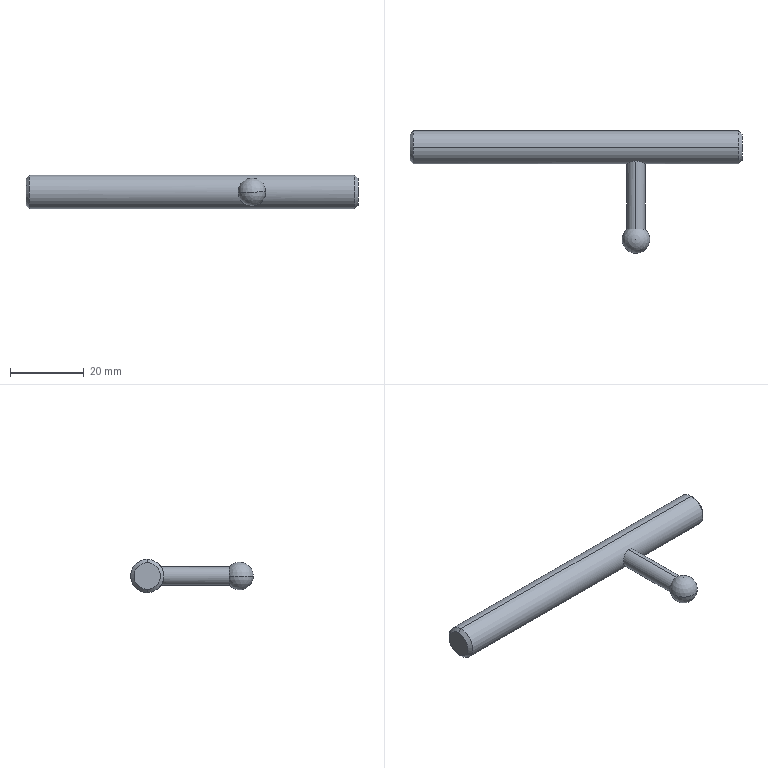Part | SolidWorks | features BaseBody 1 | 1 solid | 12 faces | box 90 x 33.25 x 9 mm | volume 6266 mm3 | cylinder 4 | cone 4 | sphere 2 | plane 2 | commonest cylinder face diameters 5 x2 9 x2
STEP:
#1=CARTESIAN_POINT('',(37.5,-25.,5.7));
#2=VERTEX_POINT('',#1);
#3=CARTESIAN_POINT('',(45.,-25.,5.7));
#4=VERTEX_POINT('',#3);
#5=CARTESIAN_POINT('',(41.25,-25.,5.7));
#6=DIRECTION('',(0.,0.,1.));
#7=DIRECTION('',(1.,0.,0.));
#8=AXIS2_PLACEMENT_3D('',#5,#6,#7);
#9=CIRCLE('',#8,3.75);
#10=EDGE_CURVE('',#2,#4,#9,.T.);
#11=ORIENTED_EDGE('',*,*,#10,.F.);
#12=CARTESIAN_POINT('',(38.75,-22.205,5.7));
#13=VERTEX_POINT('',#12);
#14=CARTESIAN_POINT('',(41.25,-25.,5.7));
#15=DIRECTION('',(0.,0.,-1.));
#16=DIRECTION('',(-1.,0.,0.));
#17=AXIS2_PLACEMENT_3D('',#14,#15,#16);
#18=CIRCLE('',#17,3.75);
#19=EDGE_CURVE('',#2,#13,#18,.T.);
#20=ORIENTED_EDGE('',*,*,#19,.T.);
#21=CARTESIAN_POINT('',(41.25,-22.205,3.2));
#22=VERTEX_POINT('',#21);
#23=CARTESIAN_POINT('',(41.25,-22.205,5.7));
#24=DIRECTION('',(0.,1.,0.));
#25=DIRECTION('',(0.,0.,-1.));
#26=AXIS2_PLACEMENT_3D('',#23,#24,#25);
#27=CIRCLE('',#26,2.5);
#28=EDGE_CURVE('',#22,#13,#27,.T.);
#29=ORIENTED_EDGE('',*,*,#28,.F.);
#30=CARTESIAN_POINT('',(43.75,-22.205,5.7));
#31=VERTEX_POINT('',#30);
#32=CARTESIAN_POINT('',(41.25,-22.205,5.7));
#33=DIRECTION('',(0.,1.,0.));
#34=DIRECTION('',(0.,0.,-1.));
#35=AXIS2_PLACEMENT_3D('',#32,#33,#34);
#36=CIRCLE('',#35,2.5);
#37=EDGE_CURVE('',#31,#22,#36,.T.);
#38=ORIENTED_EDGE('',*,*,#37,.F.);
#39=CARTESIAN_POINT('',(41.25,-25.,5.7));
#40=DIRECTION('',(0.,0.,-1.));
#41=DIRECTION('',(-1.,0.,0.));
#42=AXIS2_PLACEMENT_3D('',#39,#40,#41);
#43=CIRCLE('',#42,3.75);
#44=EDGE_CURVE('',#31,#4,#43,.T.);
#45=ORIENTED_EDGE('',*,*,#44,.T.);
#46=EDGE_LOOP('',(#11,#20,#29,#38,#45));
#47=FACE_OUTER_BOUND('',#46,.T.);
#48=CARTESIAN_POINT('',(41.25,-25.,5.7));
#49=DIRECTION('',(0.,0.,-1.));
#50=DIRECTION('',(0.,-1.,0.));
#51=AXIS2_PLACEMENT_3D('',#48,#49,#50);
#52=SPHERICAL_SURFACE('',#51,3.75);
#53=ADVANCED_FACE('',(#47),#52,.T.);
#54=CARTESIAN_POINT('',(-19.1,0.,1.2));
#55=VERTEX_POINT('',#54);
#56=CARTESIAN_POINT('',(-19.1,0.,10.2));
#57=VERTEX_POINT('',#56);
#58=CARTESIAN_POINT('',(-19.1,0.,5.7));
#59=DIRECTION('',(1.,0.,0.));
#60=DIRECTION('',(0.,0.,-1.));
#61=AXIS2_PLACEMENT_3D('',#58,#59,#60);
#62=CIRCLE('',#61,4.5);
#63=EDGE_CURVE('',#55,#57,#62,.T.);
#64=ORIENTED_EDGE('',*,*,#63,.T.);
#65=CARTESIAN_POINT('',(69.1,0.,10.2));
#66=VERTEX_POINT('',#65);
#67=CARTESIAN_POINT('',(25.,0.,10.2));
#68=DIRECTION('',(1.,0.,0.));
#69=VECTOR('',#68,1000.);
#70=LINE('',#67,#69);
#71=EDGE_CURVE('',#57,#66,#70,.T.);
#72=ORIENTED_EDGE('',*,*,#71,.T.);
#73=CARTESIAN_POINT('',(69.1,0.,1.2));
#74=VERTEX_POINT('',#73);
#75=CARTESIAN_POINT('',(69.1,0.,5.7));
#76=DIRECTION('',(-1.,0.,0.));
#77=DIRECTION('',(0.,0.,-1.));
#78=AXIS2_PLACEMENT_3D('',#75,#76,#77);
#79=CIRCLE('',#78,4.5);
#80=EDGE_CURVE('',#66,#74,#79,.T.);
#81=ORIENTED_EDGE('',*,*,#80,.T.);
#82=CARTESIAN_POINT('',(25.,0.,1.2));
#83=DIRECTION('',(1.,0.,0.));
#84=VECTOR('',#83,1000.);
#85=LINE('',#82,#84);
#86=EDGE_CURVE('',#55,#74,#85,.T.);
#87=ORIENTED_EDGE('',*,*,#86,.F.);
#88=EDGE_LOOP('',(#64,#72,#81,#87));
#89=FACE_OUTER_BOUND('',#88,.T.);
#90=CARTESIAN_POINT('',(25.,0.,5.7));
#91=DIRECTION('',(1.,0.,0.));
#92=DIRECTION('',(0.,0.,-1.));
#93=AXIS2_PLACEMENT_3D('',#90,#91,#92);
#94=CYLINDRICAL_SURFACE('',#93,4.5);
#95=ADVANCED_FACE('',(#89),#94,.T.);
#96=CARTESIAN_POINT('',(70.,0.,9.3));
#97=VERTEX_POINT('',#96);
#98=CARTESIAN_POINT('',(70.,0.,2.1));
#99=VERTEX_POINT('',#98);
#100=CARTESIAN_POINT('',(70.,0.,5.7));
#101=DIRECTION('',(-1.,0.,0.));
#102=DIRECTION('',(0.,0.,1.));
#103=AXIS2_PLACEMENT_3D('',#100,#101,#102);
#104=CIRCLE('',#103,3.6);
#105=EDGE_CURVE('',#97,#99,#104,.T.);
#106=ORIENTED_EDGE('',*,*,#105,.T.);
#107=CARTESIAN_POINT('',(69.1,0.,1.2));
#108=DIRECTION('',(-0.7071,0.,-0.7071));
#109=VECTOR('',#108,1000.);
#110=LINE('',#107,#109);
#111=EDGE_CURVE('',#99,#74,#110,.T.);
#112=ORIENTED_EDGE('',*,*,#111,.T.);
#113=ORIENTED_EDGE('',*,*,#80,.F.);
#114=CARTESIAN_POINT('',(69.1,0.,10.2));
#115=DIRECTION('',(-0.7071,0.,0.7071));
#116=VECTOR('',#115,1000.);
#117=LINE('',#114,#116);
#118=EDGE_CURVE('',#97,#66,#117,.T.);
#119=ORIENTED_EDGE('',*,*,#118,.F.);
#120=EDGE_LOOP('',(#106,#112,#113,#119));
#121=FACE_OUTER_BOUND('',#120,.T.);
#122=CARTESIAN_POINT('',(69.1,0.,5.7));
#123=DIRECTION('',(-1.,0.,0.));
#124=DIRECTION('',(0.,0.,1.));
#125=AXIS2_PLACEMENT_3D('',#122,#123,#124);
#126=CONICAL_SURFACE('',#125,4.5,0.7854);
#127=ADVANCED_FACE('',(#121),#126,.T.);
#128=CARTESIAN_POINT('',(41.25,-3.742,8.2));
#129=VERTEX_POINT('',#128);
#130=CARTESIAN_POINT('',(41.25,-3.742,3.2));
#131=VERTEX_POINT('',#130);
#132=CARTESIAN_POINT('',(41.25,-3.742,8.2));
#133=CARTESIAN_POINT('',(41.419,-3.742,8.2));
#134=CARTESIAN_POINT('',(41.584,-3.753,8.183));
#135=CARTESIAN_POINT('',(41.908,-3.796,8.117));
#136=CARTESIAN_POINT('',(42.068,-3.827,8.068));
#137=CARTESIAN_POINT('',(42.519,-3.94,7.879));
#138=CARTESIAN_POINT('',(42.789,-4.041,7.695));
#139=CARTESIAN_POINT('',(43.128,-4.185,7.357));
#140=CARTESIAN_POINT('',(43.232,-4.233,7.232));
#141=CARTESIAN_POINT('',(43.413,-4.321,6.964));
#142=CARTESIAN_POINT('',(43.49,-4.36,6.823));
#143=CARTESIAN_POINT('',(43.617,-4.427,6.522));
#144=CARTESIAN_POINT('',(43.667,-4.454,6.362));
#145=CARTESIAN_POINT('',(43.733,-4.49,6.037));
#146=CARTESIAN_POINT('',(43.75,-4.5,5.872));
#147=CARTESIAN_POINT('',(43.75,-4.5,5.537));
#148=CARTESIAN_POINT('',(43.733,-4.491,5.368));
#149=CARTESIAN_POINT('',(43.668,-4.455,5.043));
#150=CARTESIAN_POINT('',(43.618,-4.428,4.883));
#151=CARTESIAN_POINT('',(43.491,-4.361,4.58));
#152=CARTESIAN_POINT('',(43.414,-4.322,4.437));
#153=CARTESIAN_POINT('',(43.233,-4.234,4.169));
#154=CARTESIAN_POINT('',(43.129,-4.186,4.043));
#155=CARTESIAN_POINT('',(42.79,-4.041,3.705));
#156=CARTESIAN_POINT('',(42.519,-3.94,3.522));
#157=CARTESIAN_POINT('',(42.071,-3.828,3.333));
#158=CARTESIAN_POINT('',(41.912,-3.796,3.283));
#159=CARTESIAN_POINT('',(41.585,-3.753,3.217));
#160=CARTESIAN_POINT('',(41.419,-3.742,3.2));
#161=CARTESIAN_POINT('',(41.25,-3.742,3.2));
#162=B_SPLINE_CURVE_WITH_KNOTS('',3,(#132,#133,#134,#135,#136,#137,#138,#139,#140,#141,#142,#143,#144,#145,#146,#147,#148,#149,#150,#151,#152,#153,#154,#155,#156,#157,#158,#159,#160,#161),.UNSPECIFIED.,.F.,.F.,(4,2,2,2,2,2,2,2,2,2,2,2,2,2,4),(0.,0.000499,0.0009979,0.001996,0.002495,0.002994,0.003493,0.003992,0.004491,0.00499,0.005489,0.005988,0.006985,0.007484,0.007983),.UNSPECIFIED.);
#163=EDGE_CURVE('',#129,#131,#162,.T.);
#164=ORIENTED_EDGE('',*,*,#163,.F.);
#165=CARTESIAN_POINT('',(41.25,-22.205,8.2));
#166=VERTEX_POINT('',#165);
#167=CARTESIAN_POINT('',(41.25,-12.5,8.2));
#168=DIRECTION('',(0.,-1.,0.));
#169=VECTOR('',#168,1000.);
#170=LINE('',#167,#169);
#171=EDGE_CURVE('',#129,#166,#170,.T.);
#172=ORIENTED_EDGE('',*,*,#171,.T.);
#173=CARTESIAN_POINT('',(41.25,-22.205,5.7));
#174=DIRECTION('',(0.,1.,0.));
#175=DIRECTION('',(0.,0.,-1.));
#176=AXIS2_PLACEMENT_3D('',#173,#174,#175);
#177=CIRCLE('',#176,2.5);
#178=EDGE_CURVE('',#166,#31,#177,.T.);
#179=ORIENTED_EDGE('',*,*,#178,.T.);
#180=ORIENTED_EDGE('',*,*,#37,.T.);
#181=CARTESIAN_POINT('',(41.25,-12.5,3.2));
#182=DIRECTION('',(0.,-1.,0.));
#183=VECTOR('',#182,1000.);
#184=LINE('',#181,#183);
#185=EDGE_CURVE('',#131,#22,#184,.T.);
#186=ORIENTED_EDGE('',*,*,#185,.F.);
#187=EDGE_LOOP('',(#164,#172,#179,#180,#186));
#188=FACE_OUTER_BOUND('',#187,.T.);
#189=CARTESIAN_POINT('',(41.25,-12.5,5.7));
#190=DIRECTION('',(0.,-1.,0.));
#191=DIRECTION('',(0.,0.,-1.));
#192=AXIS2_PLACEMENT_3D('',#189,#190,#191);
#193=CYLINDRICAL_SURFACE('',#192,2.5);
#194=ADVANCED_FACE('',(#188),#193,.T.);
#195=CARTESIAN_POINT('',(-20.,0.,2.1));
#196=VERTEX_POINT('',#195);
#197=CARTESIAN_POINT('',(-20.,0.,9.3));
#198=VERTEX_POINT('',#197);
#199=CARTESIAN_POINT('',(-20.,0.,5.7));
#200=DIRECTION('',(1.,0.,0.));
#201=DIRECTION('',(0.,0.,-1.));
#202=AXIS2_PLACEMENT_3D('',#199,#200,#201);
#203=CIRCLE('',#202,3.6);
#204=EDGE_CURVE('',#196,#198,#203,.T.);
#205=ORIENTED_EDGE('',*,*,#204,.T.);
#206=CARTESIAN_POINT('',(-19.1,0.,10.2));
#207=DIRECTION('',(0.7071,0.,0.7071));
#208=VECTOR('',#207,1000.);
#209=LINE('',#206,#208);
#210=EDGE_CURVE('',#198,#57,#209,.T.);
#211=ORIENTED_EDGE('',*,*,#210,.T.);
#212=ORIENTED_EDGE('',*,*,#63,.F.);
#213=CARTESIAN_POINT('',(-19.1,0.,1.2));
#214=DIRECTION('',(0.7071,0.,-0.7071));
#215=VECTOR('',#214,1000.);
#216=LINE('',#213,#215);
#217=EDGE_CURVE('',#196,#55,#216,.T.);
#218=ORIENTED_EDGE('',*,*,#217,.F.);
#219=EDGE_LOOP('',(#205,#211,#212,#218));
#220=FACE_OUTER_BOUND('',#219,.T.);
#221=CARTESIAN_POINT('',(-19.1,0.,5.7));
#222=DIRECTION('',(1.,0.,0.));
#223=DIRECTION('',(0.,0.,-1.));
#224=AXIS2_PLACEMENT_3D('',#221,#222,#223);
#225=CONICAL_SURFACE('',#224,4.5,0.7854);
#226=ADVANCED_FACE('',(#220),#225,.T.);
#227=ORIENTED_EDGE('',*,*,#204,.F.);
#228=CARTESIAN_POINT('',(-20.,0.,5.7));
#229=DIRECTION('',(1.,0.,0.));
#230=DIRECTION('',(0.,0.,-1.));
#231=AXIS2_PLACEMENT_3D('',#228,#229,#230);
#232=CIRCLE('',#231,3.6);
#233=EDGE_CURVE('',#198,#196,#232,.T.);
#234=ORIENTED_EDGE('',*,*,#233,.F.);
#235=EDGE_LOOP('',(#227,#234));
#236=FACE_OUTER_BOUND('',#235,.T.);
#237=CARTESIAN_POINT('',(-20.,1.8,5.7));
#238=DIRECTION('',(-1.,0.,0.));
#239=DIRECTION('',(0.,0.,1.));
#240=AXIS2_PLACEMENT_3D('',#237,#238,#239);
#241=PLANE('',#240);
#242=ADVANCED_FACE('',(#236),#241,.T.);
#243=ORIENTED_EDGE('',*,*,#105,.F.);
#244=CARTESIAN_POINT('',(70.,0.,5.7));
#245=DIRECTION('',(-1.,0.,0.));
#246=DIRECTION('',(0.,0.,1.));
#247=AXIS2_PLACEMENT_3D('',#244,#245,#246);
#248=CIRCLE('',#247,3.6);
#249=EDGE_CURVE('',#99,#97,#248,.T.);
#250=ORIENTED_EDGE('',*,*,#249,.F.);
#251=EDGE_LOOP('',(#243,#250));
#252=FACE_OUTER_BOUND('',#251,.T.);
#253=CARTESIAN_POINT('',(70.,1.8,5.7));
#254=DIRECTION('',(1.,0.,0.));
#255=DIRECTION('',(0.,1.,0.));
#256=AXIS2_PLACEMENT_3D('',#253,#254,#255);
#257=PLANE('',#256);
#258=ADVANCED_FACE('',(#252),#257,.T.);
#259=ORIENTED_EDGE('',*,*,#210,.F.);
#260=ORIENTED_EDGE('',*,*,#233,.T.);
#261=ORIENTED_EDGE('',*,*,#217,.T.);
#262=CARTESIAN_POINT('',(-19.1,0.,5.7));
#263=DIRECTION('',(1.,0.,0.));
#264=DIRECTION('',(0.,0.,-1.));
#265=AXIS2_PLACEMENT_3D('',#262,#263,#264);
#266=CIRCLE('',#265,4.5);
#267=EDGE_CURVE('',#57,#55,#266,.T.);
#268=ORIENTED_EDGE('',*,*,#267,.F.);
#269=EDGE_LOOP('',(#259,#260,#261,#268));
#270=FACE_OUTER_BOUND('',#269,.T.);
#271=CARTESIAN_POINT('',(-19.1,0.,5.7));
#272=DIRECTION('',(1.,0.,0.));
#273=DIRECTION('',(0.,0.,-1.));
#274=AXIS2_PLACEMENT_3D('',#271,#272,#273);
#275=CONICAL_SURFACE('',#274,4.5,0.7854);
#276=ADVANCED_FACE('',(#270),#275,.T.);
#277=ORIENTED_EDGE('',*,*,#171,.F.);
#278=CARTESIAN_POINT('',(41.25,-3.742,3.2));
#279=CARTESIAN_POINT('',(41.081,-3.742,3.2));
#280=CARTESIAN_POINT('',(40.916,-3.753,3.217));
#281=CARTESIAN_POINT('',(40.592,-3.796,3.283));
#282=CARTESIAN_POINT('',(40.432,-3.827,3.332));
#283=CARTESIAN_POINT('',(39.981,-3.94,3.521));
#284=CARTESIAN_POINT('',(39.711,-4.041,3.705));
#285=CARTESIAN_POINT('',(39.372,-4.185,4.043));
#286=CARTESIAN_POINT('',(39.268,-4.233,4.168));
#287=CARTESIAN_POINT('',(39.087,-4.321,4.436));
#288=CARTESIAN_POINT('',(39.01,-4.36,4.577));
#289=CARTESIAN_POINT('',(38.883,-4.427,4.878));
#290=CARTESIAN_POINT('',(38.833,-4.454,5.038));
#291=CARTESIAN_POINT('',(38.767,-4.49,5.363));
#292=CARTESIAN_POINT('',(38.75,-4.5,5.528));
#293=CARTESIAN_POINT('',(38.75,-4.5,5.863));
#294=CARTESIAN_POINT('',(38.767,-4.491,6.032));
#295=CARTESIAN_POINT('',(38.832,-4.455,6.357));
#296=CARTESIAN_POINT('',(38.882,-4.428,6.517));
#297=CARTESIAN_POINT('',(39.009,-4.361,6.82));
#298=CARTESIAN_POINT('',(39.086,-4.322,6.963));
#299=CARTESIAN_POINT('',(39.267,-4.234,7.231));
#300=CARTESIAN_POINT('',(39.371,-4.186,7.357));
#301=CARTESIAN_POINT('',(39.71,-4.041,7.695));
#302=CARTESIAN_POINT('',(39.981,-3.94,7.878));
#303=CARTESIAN_POINT('',(40.429,-3.828,8.067));
#304=CARTESIAN_POINT('',(40.588,-3.796,8.117));
#305=CARTESIAN_POINT('',(40.915,-3.753,8.183));
#306=CARTESIAN_POINT('',(41.081,-3.742,8.2));
#307=CARTESIAN_POINT('',(41.25,-3.742,8.2));
#308=B_SPLINE_CURVE_WITH_KNOTS('',3,(#278,#279,#280,#281,#282,#283,#284,#285,#286,#287,#288,#289,#290,#291,#292,#293,#294,#295,#296,#297,#298,#299,#300,#301,#302,#303,#304,#305,#306,#307),.UNSPECIFIED.,.F.,.F.,(4,2,2,2,2,2,2,2,2,2,2,2,2,2,4),(0.007983,0.008482,0.00898,0.009977,0.01048,0.01097,0.01147,0.01197,0.01247,0.01297,0.01347,0.01396,0.01496,0.01546,0.01596),.UNSPECIFIED.);
#309=EDGE_CURVE('',#131,#129,#308,.T.);
#310=ORIENTED_EDGE('',*,*,#309,.F.);
#311=ORIENTED_EDGE('',*,*,#185,.T.);
#312=ORIENTED_EDGE('',*,*,#28,.T.);
#313=CARTESIAN_POINT('',(41.25,-22.205,5.7));
#314=DIRECTION('',(0.,1.,0.));
#315=DIRECTION('',(0.,0.,-1.));
#316=AXIS2_PLACEMENT_3D('',#313,#314,#315);
#317=CIRCLE('',#316,2.5);
#318=EDGE_CURVE('',#13,#166,#317,.T.);
#319=ORIENTED_EDGE('',*,*,#318,.T.);
#320=EDGE_LOOP('',(#277,#310,#311,#312,#319));
#321=FACE_OUTER_BOUND('',#320,.T.);
#322=CARTESIAN_POINT('',(41.25,-12.5,5.7));
#323=DIRECTION('',(0.,-1.,0.));
#324=DIRECTION('',(0.,0.,-1.));
#325=AXIS2_PLACEMENT_3D('',#322,#323,#324);
#326=CYLINDRICAL_SURFACE('',#325,2.5);
#327=ADVANCED_FACE('',(#321),#326,.T.);
#328=ORIENTED_EDGE('',*,*,#111,.F.);
#329=ORIENTED_EDGE('',*,*,#249,.T.);
#330=ORIENTED_EDGE('',*,*,#118,.T.);
#331=CARTESIAN_POINT('',(69.1,0.,5.7));
#332=DIRECTION('',(-1.,0.,0.));
#333=DIRECTION('',(0.,0.,-1.));
#334=AXIS2_PLACEMENT_3D('',#331,#332,#333);
#335=CIRCLE('',#334,4.5);
#336=EDGE_CURVE('',#74,#66,#335,.T.);
#337=ORIENTED_EDGE('',*,*,#336,.F.);
#338=EDGE_LOOP('',(#328,#329,#330,#337));
#339=FACE_OUTER_BOUND('',#338,.T.);
#340=CARTESIAN_POINT('',(69.1,0.,5.7));
#341=DIRECTION('',(-1.,0.,0.));
#342=DIRECTION('',(0.,0.,1.));
#343=AXIS2_PLACEMENT_3D('',#340,#341,#342);
#344=CONICAL_SURFACE('',#343,4.5,0.7854);
#345=ADVANCED_FACE('',(#339),#344,.T.);
#346=ORIENTED_EDGE('',*,*,#71,.F.);
#347=ORIENTED_EDGE('',*,*,#267,.T.);
#348=ORIENTED_EDGE('',*,*,#86,.T.);
#349=ORIENTED_EDGE('',*,*,#336,.T.);
#350=EDGE_LOOP('',(#346,#347,#348,#349));
#351=FACE_OUTER_BOUND('',#350,.T.);
#352=ORIENTED_EDGE('',*,*,#309,.T.);
#353=ORIENTED_EDGE('',*,*,#163,.T.);
#354=EDGE_LOOP('',(#352,#353));
#355=FACE_BOUND('',#354,.T.);
#356=CARTESIAN_POINT('',(25.,0.,5.7));
#357=DIRECTION('',(1.,0.,0.));
#358=DIRECTION('',(0.,0.,-1.));
#359=AXIS2_PLACEMENT_3D('',#356,#357,#358);
#360=CYLINDRICAL_SURFACE('',#359,4.5);
#361=ADVANCED_FACE('',(#351,#355),#360,.T.);
#362=ORIENTED_EDGE('',*,*,#19,.F.);
#363=ORIENTED_EDGE('',*,*,#10,.T.);
#364=ORIENTED_EDGE('',*,*,#44,.F.);
#365=ORIENTED_EDGE('',*,*,#178,.F.);
#366=ORIENTED_EDGE('',*,*,#318,.F.);
#367=EDGE_LOOP('',(#362,#363,#364,#365,#366));
#368=FACE_OUTER_BOUND('',#367,.T.);
#369=CARTESIAN_POINT('',(41.25,-25.,5.7));
#370=DIRECTION('',(0.,0.,-1.));
#371=DIRECTION('',(0.,-1.,0.));
#372=AXIS2_PLACEMENT_3D('',#369,#370,#371);
#373=SPHERICAL_SURFACE('',#372,3.75);
#374=ADVANCED_FACE('',(#368),#373,.T.);
#375=CLOSED_SHELL('',(#53,#95,#127,#194,#226,#242,#258,#276,#327,#345,#361,#374));
#376=MANIFOLD_SOLID_BREP('',#375);
#377=CARTESIAN_POINT('',(0.,0.,0.));
#378=DIRECTION('',(0.,0.,1.));
#379=DIRECTION('',(1.,0.,0.));
#380=AXIS2_PLACEMENT_3D('',#377,#378,#379);
#381=(LENGTH_UNIT()NAMED_UNIT(*)SI_UNIT(.MILLI.,.METRE.));
#382=UNCERTAINTY_MEASURE_WITH_UNIT(LENGTH_MEASURE(0.00001),#381,'','');
#383=(NAMED_UNIT(*)PLANE_ANGLE_UNIT()SI_UNIT($,.RADIAN.));
#384=(NAMED_UNIT(*)SI_UNIT($,.STERADIAN.)SOLID_ANGLE_UNIT());
#385=(GEOMETRIC_REPRESENTATION_CONTEXT(3)GLOBAL_UNCERTAINTY_ASSIGNED_CONTEXT((#382))GLOBAL_UNIT_ASSIGNED_CONTEXT((#381,#383,#384))REPRESENTATION_CONTEXT('',''));
#386=ADVANCED_BREP_SHAPE_REPRESENTATION('',(#376,#380),#385);